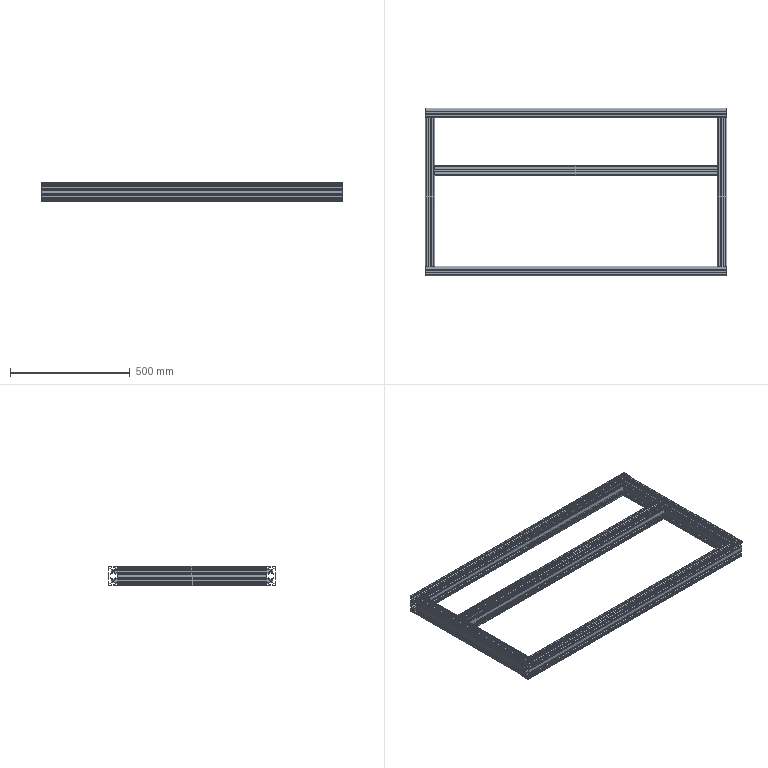Part | SolidWorks | features 3DProfileFeature 1, ICE 1, WeldCornerFeat 1, WeldMemberFeat 1, WeldmentFeature 1 | 5 solids | 1220 faces | box 1260 x 700.002 x 80 mm | volume 4888550 mm3 | plane 1145 | cylinder 75 | commonest cylinder face diameters 9 x35 5 x20 6.8 x20